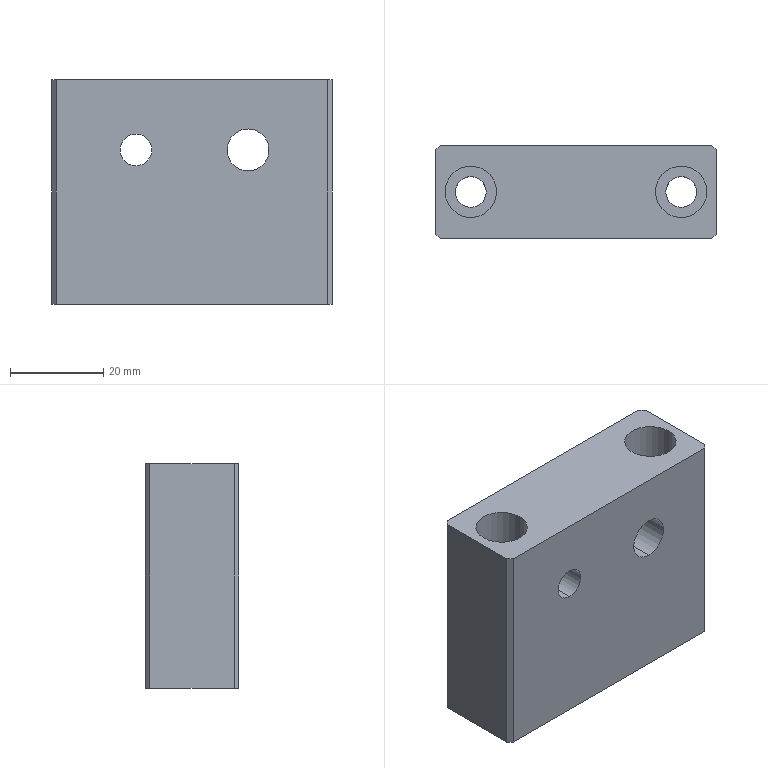Part | SolidWorks | features HoleWzd 3, Chamfer 1, Extrusion 1 | 1 solid | 24 faces | box 60 x 20 x 48 mm | volume 51248 mm3 | cylinder 12 | plane 12 | commonest cylinder face diameters 6.6 x4 11 x4 6.8 x2 9 x2
STEP:
#1=CARTESIAN_POINT('',(12.,10.,37.5));
#2=VERTEX_POINT('',#1);
#3=CARTESIAN_POINT('',(12.,10.,28.5));
#4=VERTEX_POINT('',#3);
#5=CARTESIAN_POINT('',(12.,10.,33.));
#6=DIRECTION('',(0.,-1.,0.));
#7=DIRECTION('',(0.,0.,-1.));
#8=AXIS2_PLACEMENT_3D('',#5,#6,#7);
#9=CIRCLE('',#8,4.5);
#10=EDGE_CURVE('',#2,#4,#9,.T.);
#11=ORIENTED_EDGE('',*,*,#10,.F.);
#12=CARTESIAN_POINT('',(12.,-10.,37.5));
#13=VERTEX_POINT('',#12);
#14=CARTESIAN_POINT('',(12.,-10.,37.5));
#15=DIRECTION('',(0.,-1.,0.));
#16=VECTOR('',#15,1000.);
#17=LINE('',#14,#16);
#18=EDGE_CURVE('',#2,#13,#17,.T.);
#19=ORIENTED_EDGE('',*,*,#18,.T.);
#20=CARTESIAN_POINT('',(12.,-10.,28.5));
#21=VERTEX_POINT('',#20);
#22=CARTESIAN_POINT('',(12.,-10.,33.));
#23=DIRECTION('',(0.,-1.,0.));
#24=DIRECTION('',(0.,0.,-1.));
#25=AXIS2_PLACEMENT_3D('',#22,#23,#24);
#26=CIRCLE('',#25,4.5);
#27=EDGE_CURVE('',#13,#21,#26,.T.);
#28=ORIENTED_EDGE('',*,*,#27,.T.);
#29=CARTESIAN_POINT('',(12.,-10.,28.5));
#30=DIRECTION('',(0.,-1.,0.));
#31=VECTOR('',#30,1000.);
#32=LINE('',#29,#31);
#33=EDGE_CURVE('',#4,#21,#32,.T.);
#34=ORIENTED_EDGE('',*,*,#33,.F.);
#35=EDGE_LOOP('',(#11,#19,#28,#34));
#36=FACE_OUTER_BOUND('',#35,.T.);
#37=CARTESIAN_POINT('',(12.,-10.,33.));
#38=DIRECTION('',(0.,-1.,0.));
#39=DIRECTION('',(0.,0.,-1.));
#40=AXIS2_PLACEMENT_3D('',#37,#38,#39);
#41=CYLINDRICAL_SURFACE('',#40,4.5);
#42=ADVANCED_FACE('',(#36),#41,.F.);
#43=CARTESIAN_POINT('',(-12.,10.,36.4));
#44=VERTEX_POINT('',#43);
#45=CARTESIAN_POINT('',(-12.,10.,29.6));
#46=VERTEX_POINT('',#45);
#47=CARTESIAN_POINT('',(-12.,10.,33.));
#48=DIRECTION('',(0.,-1.,0.));
#49=DIRECTION('',(0.,0.,-1.));
#50=AXIS2_PLACEMENT_3D('',#47,#48,#49);
#51=CIRCLE('',#50,3.4);
#52=EDGE_CURVE('',#44,#46,#51,.T.);
#53=ORIENTED_EDGE('',*,*,#52,.F.);
#54=CARTESIAN_POINT('',(-12.,-10.,36.4));
#55=VERTEX_POINT('',#54);
#56=CARTESIAN_POINT('',(-12.,-10.,36.4));
#57=DIRECTION('',(0.,-1.,0.));
#58=VECTOR('',#57,1000.);
#59=LINE('',#56,#58);
#60=EDGE_CURVE('',#44,#55,#59,.T.);
#61=ORIENTED_EDGE('',*,*,#60,.T.);
#62=CARTESIAN_POINT('',(-12.,-10.,29.6));
#63=VERTEX_POINT('',#62);
#64=CARTESIAN_POINT('',(-12.,-10.,33.));
#65=DIRECTION('',(0.,-1.,0.));
#66=DIRECTION('',(0.,0.,-1.));
#67=AXIS2_PLACEMENT_3D('',#64,#65,#66);
#68=CIRCLE('',#67,3.4);
#69=EDGE_CURVE('',#55,#63,#68,.T.);
#70=ORIENTED_EDGE('',*,*,#69,.T.);
#71=CARTESIAN_POINT('',(-12.,-10.,29.6));
#72=DIRECTION('',(0.,-1.,0.));
#73=VECTOR('',#72,1000.);
#74=LINE('',#71,#73);
#75=EDGE_CURVE('',#46,#63,#74,.T.);
#76=ORIENTED_EDGE('',*,*,#75,.F.);
#77=EDGE_LOOP('',(#53,#61,#70,#76));
#78=FACE_OUTER_BOUND('',#77,.T.);
#79=CARTESIAN_POINT('',(-12.,-10.,33.));
#80=DIRECTION('',(0.,-1.,0.));
#81=DIRECTION('',(0.,0.,-1.));
#82=AXIS2_PLACEMENT_3D('',#79,#80,#81);
#83=CYLINDRICAL_SURFACE('',#82,3.4);
#84=ADVANCED_FACE('',(#78),#83,.F.);
#85=CARTESIAN_POINT('',(-28.,0.,40.));
#86=VERTEX_POINT('',#85);
#87=CARTESIAN_POINT('',(-17.,0.,40.));
#88=VERTEX_POINT('',#87);
#89=CARTESIAN_POINT('',(-22.5,0.,40.));
#90=DIRECTION('',(0.,0.,1.));
#91=DIRECTION('',(1.,0.,0.));
#92=AXIS2_PLACEMENT_3D('',#89,#90,#91);
#93=CIRCLE('',#92,5.5);
#94=EDGE_CURVE('',#86,#88,#93,.T.);
#95=ORIENTED_EDGE('',*,*,#94,.F.);
#96=CARTESIAN_POINT('',(-28.,0.,48.));
#97=VERTEX_POINT('',#96);
#98=CARTESIAN_POINT('',(-28.,0.,48.));
#99=DIRECTION('',(0.,0.,1.));
#100=VECTOR('',#99,1000.);
#101=LINE('',#98,#100);
#102=EDGE_CURVE('',#86,#97,#101,.T.);
#103=ORIENTED_EDGE('',*,*,#102,.T.);
#104=CARTESIAN_POINT('',(-17.,0.,48.));
#105=VERTEX_POINT('',#104);
#106=CARTESIAN_POINT('',(-22.5,0.,48.));
#107=DIRECTION('',(0.,0.,1.));
#108=DIRECTION('',(1.,0.,0.));
#109=AXIS2_PLACEMENT_3D('',#106,#107,#108);
#110=CIRCLE('',#109,5.5);
#111=EDGE_CURVE('',#97,#105,#110,.T.);
#112=ORIENTED_EDGE('',*,*,#111,.T.);
#113=CARTESIAN_POINT('',(-17.,0.,48.));
#114=DIRECTION('',(0.,0.,1.));
#115=VECTOR('',#114,1000.);
#116=LINE('',#113,#115);
#117=EDGE_CURVE('',#88,#105,#116,.T.);
#118=ORIENTED_EDGE('',*,*,#117,.F.);
#119=EDGE_LOOP('',(#95,#103,#112,#118));
#120=FACE_OUTER_BOUND('',#119,.T.);
#121=CARTESIAN_POINT('',(-22.5,0.,48.));
#122=DIRECTION('',(0.,0.,1.));
#123=DIRECTION('',(1.,0.,0.));
#124=AXIS2_PLACEMENT_3D('',#121,#122,#123);
#125=CYLINDRICAL_SURFACE('',#124,5.5);
#126=ADVANCED_FACE('',(#120),#125,.F.);
#127=CARTESIAN_POINT('',(-25.8,0.,0.));
#128=VERTEX_POINT('',#127);
#129=CARTESIAN_POINT('',(-19.2,0.,0.));
#130=VERTEX_POINT('',#129);
#131=CARTESIAN_POINT('',(-22.5,0.,0.));
#132=DIRECTION('',(0.,0.,1.));
#133=DIRECTION('',(1.,0.,0.));
#134=AXIS2_PLACEMENT_3D('',#131,#132,#133);
#135=CIRCLE('',#134,3.3);
#136=EDGE_CURVE('',#128,#130,#135,.T.);
#137=ORIENTED_EDGE('',*,*,#136,.F.);
#138=CARTESIAN_POINT('',(-25.8,0.,40.));
#139=VERTEX_POINT('',#138);
#140=CARTESIAN_POINT('',(-25.8,0.,48.));
#141=DIRECTION('',(0.,0.,1.));
#142=VECTOR('',#141,1000.);
#143=LINE('',#140,#142);
#144=EDGE_CURVE('',#128,#139,#143,.T.);
#145=ORIENTED_EDGE('',*,*,#144,.T.);
#146=CARTESIAN_POINT('',(-19.2,0.,40.));
#147=VERTEX_POINT('',#146);
#148=CARTESIAN_POINT('',(-22.5,0.,40.));
#149=DIRECTION('',(0.,0.,1.));
#150=DIRECTION('',(1.,0.,0.));
#151=AXIS2_PLACEMENT_3D('',#148,#149,#150);
#152=CIRCLE('',#151,3.3);
#153=EDGE_CURVE('',#139,#147,#152,.T.);
#154=ORIENTED_EDGE('',*,*,#153,.T.);
#155=CARTESIAN_POINT('',(-19.2,0.,48.));
#156=DIRECTION('',(0.,0.,1.));
#157=VECTOR('',#156,1000.);
#158=LINE('',#155,#157);
#159=EDGE_CURVE('',#130,#147,#158,.T.);
#160=ORIENTED_EDGE('',*,*,#159,.F.);
#161=EDGE_LOOP('',(#137,#145,#154,#160));
#162=FACE_OUTER_BOUND('',#161,.T.);
#163=CARTESIAN_POINT('',(-22.5,0.,48.));
#164=DIRECTION('',(0.,0.,1.));
#165=DIRECTION('',(1.,0.,0.));
#166=AXIS2_PLACEMENT_3D('',#163,#164,#165);
#167=CYLINDRICAL_SURFACE('',#166,3.3);
#168=ADVANCED_FACE('',(#162),#167,.F.);
#169=CARTESIAN_POINT('',(17.,0.,40.));
#170=VERTEX_POINT('',#169);
#171=CARTESIAN_POINT('',(28.,0.,40.));
#172=VERTEX_POINT('',#171);
#173=CARTESIAN_POINT('',(22.5,0.,40.));
#174=DIRECTION('',(0.,0.,1.));
#175=DIRECTION('',(1.,0.,0.));
#176=AXIS2_PLACEMENT_3D('',#173,#174,#175);
#177=CIRCLE('',#176,5.5);
#178=EDGE_CURVE('',#170,#172,#177,.T.);
#179=ORIENTED_EDGE('',*,*,#178,.F.);
#180=CARTESIAN_POINT('',(17.,0.,48.));
#181=VERTEX_POINT('',#180);
#182=CARTESIAN_POINT('',(17.,0.,48.));
#183=DIRECTION('',(0.,0.,1.));
#184=VECTOR('',#183,1000.);
#185=LINE('',#182,#184);
#186=EDGE_CURVE('',#170,#181,#185,.T.);
#187=ORIENTED_EDGE('',*,*,#186,.T.);
#188=CARTESIAN_POINT('',(28.,0.,48.));
#189=VERTEX_POINT('',#188);
#190=CARTESIAN_POINT('',(22.5,0.,48.));
#191=DIRECTION('',(0.,0.,1.));
#192=DIRECTION('',(1.,0.,0.));
#193=AXIS2_PLACEMENT_3D('',#190,#191,#192);
#194=CIRCLE('',#193,5.5);
#195=EDGE_CURVE('',#181,#189,#194,.T.);
#196=ORIENTED_EDGE('',*,*,#195,.T.);
#197=CARTESIAN_POINT('',(28.,0.,48.));
#198=DIRECTION('',(0.,0.,1.));
#199=VECTOR('',#198,1000.);
#200=LINE('',#197,#199);
#201=EDGE_CURVE('',#172,#189,#200,.T.);
#202=ORIENTED_EDGE('',*,*,#201,.F.);
#203=EDGE_LOOP('',(#179,#187,#196,#202));
#204=FACE_OUTER_BOUND('',#203,.T.);
#205=CARTESIAN_POINT('',(22.5,0.,48.));
#206=DIRECTION('',(0.,0.,1.));
#207=DIRECTION('',(1.,0.,0.));
#208=AXIS2_PLACEMENT_3D('',#205,#206,#207);
#209=CYLINDRICAL_SURFACE('',#208,5.5);
#210=ADVANCED_FACE('',(#204),#209,.F.);
#211=CARTESIAN_POINT('',(19.2,0.,0.));
#212=VERTEX_POINT('',#211);
#213=CARTESIAN_POINT('',(25.8,0.,0.));
#214=VERTEX_POINT('',#213);
#215=CARTESIAN_POINT('',(22.5,0.,0.));
#216=DIRECTION('',(0.,0.,1.));
#217=DIRECTION('',(1.,0.,0.));
#218=AXIS2_PLACEMENT_3D('',#215,#216,#217);
#219=CIRCLE('',#218,3.3);
#220=EDGE_CURVE('',#212,#214,#219,.T.);
#221=ORIENTED_EDGE('',*,*,#220,.F.);
#222=CARTESIAN_POINT('',(19.2,0.,40.));
#223=VERTEX_POINT('',#222);
#224=CARTESIAN_POINT('',(19.2,0.,48.));
#225=DIRECTION('',(0.,0.,1.));
#226=VECTOR('',#225,1000.);
#227=LINE('',#224,#226);
#228=EDGE_CURVE('',#212,#223,#227,.T.);
#229=ORIENTED_EDGE('',*,*,#228,.T.);
#230=CARTESIAN_POINT('',(25.8,0.,40.));
#231=VERTEX_POINT('',#230);
#232=CARTESIAN_POINT('',(22.5,0.,40.));
#233=DIRECTION('',(0.,0.,1.));
#234=DIRECTION('',(1.,0.,0.));
#235=AXIS2_PLACEMENT_3D('',#232,#233,#234);
#236=CIRCLE('',#235,3.3);
#237=EDGE_CURVE('',#223,#231,#236,.T.);
#238=ORIENTED_EDGE('',*,*,#237,.T.);
#239=CARTESIAN_POINT('',(25.8,0.,48.));
#240=DIRECTION('',(0.,0.,1.));
#241=VECTOR('',#240,1000.);
#242=LINE('',#239,#241);
#243=EDGE_CURVE('',#214,#231,#242,.T.);
#244=ORIENTED_EDGE('',*,*,#243,.F.);
#245=EDGE_LOOP('',(#221,#229,#238,#244));
#246=FACE_OUTER_BOUND('',#245,.T.);
#247=CARTESIAN_POINT('',(22.5,0.,48.));
#248=DIRECTION('',(0.,0.,1.));
#249=DIRECTION('',(1.,0.,0.));
#250=AXIS2_PLACEMENT_3D('',#247,#248,#249);
#251=CYLINDRICAL_SURFACE('',#250,3.3);
#252=ADVANCED_FACE('',(#246),#251,.F.);
#253=CARTESIAN_POINT('',(-12.,-10.,33.));
#254=DIRECTION('',(0.,-1.,0.));
#255=DIRECTION('',(0.,0.,-1.));
#256=AXIS2_PLACEMENT_3D('',#253,#254,#255);
#257=CIRCLE('',#256,3.4);
#258=EDGE_CURVE('',#63,#55,#257,.T.);
#259=ORIENTED_EDGE('',*,*,#258,.F.);
#260=ORIENTED_EDGE('',*,*,#69,.F.);
#261=EDGE_LOOP('',(#259,#260));
#262=FACE_BOUND('',#261,.T.);
#263=CARTESIAN_POINT('',(-29.,-10.,0.));
#264=VERTEX_POINT('',#263);
#265=CARTESIAN_POINT('',(29.,-10.,0.));
#266=VERTEX_POINT('',#265);
#267=CARTESIAN_POINT('',(-30.,-10.,0.));
#268=DIRECTION('',(1.,0.,0.));
#269=VECTOR('',#268,1000.);
#270=LINE('',#267,#269);
#271=EDGE_CURVE('',#264,#266,#270,.T.);
#272=ORIENTED_EDGE('',*,*,#271,.T.);
#273=CARTESIAN_POINT('',(29.,-10.,48.));
#274=VERTEX_POINT('',#273);
#275=CARTESIAN_POINT('',(29.,-10.,48.));
#276=DIRECTION('',(0.,0.,1.));
#277=VECTOR('',#276,1000.);
#278=LINE('',#275,#277);
#279=EDGE_CURVE('',#266,#274,#278,.T.);
#280=ORIENTED_EDGE('',*,*,#279,.T.);
#281=CARTESIAN_POINT('',(-29.,-10.,48.));
#282=VERTEX_POINT('',#281);
#283=CARTESIAN_POINT('',(-30.,-10.,48.));
#284=DIRECTION('',(1.,0.,0.));
#285=VECTOR('',#284,1000.);
#286=LINE('',#283,#285);
#287=EDGE_CURVE('',#282,#274,#286,.T.);
#288=ORIENTED_EDGE('',*,*,#287,.F.);
#289=CARTESIAN_POINT('',(-29.,-10.,48.));
#290=DIRECTION('',(0.,0.,-1.));
#291=VECTOR('',#290,1000.);
#292=LINE('',#289,#291);
#293=EDGE_CURVE('',#282,#264,#292,.T.);
#294=ORIENTED_EDGE('',*,*,#293,.T.);
#295=EDGE_LOOP('',(#272,#280,#288,#294));
#296=FACE_OUTER_BOUND('',#295,.T.);
#297=CARTESIAN_POINT('',(12.,-10.,33.));
#298=DIRECTION('',(0.,-1.,0.));
#299=DIRECTION('',(0.,0.,-1.));
#300=AXIS2_PLACEMENT_3D('',#297,#298,#299);
#301=CIRCLE('',#300,4.5);
#302=EDGE_CURVE('',#21,#13,#301,.T.);
#303=ORIENTED_EDGE('',*,*,#302,.F.);
#304=ORIENTED_EDGE('',*,*,#27,.F.);
#305=EDGE_LOOP('',(#303,#304));
#306=FACE_BOUND('',#305,.T.);
#307=CARTESIAN_POINT('',(-30.,-10.,48.));
#308=DIRECTION('',(0.,1.,0.));
#309=DIRECTION('',(0.,0.,1.));
#310=AXIS2_PLACEMENT_3D('',#307,#308,#309);
#311=PLANE('',#310);
#312=ADVANCED_FACE('',(#262,#296,#306),#311,.F.);
#313=CARTESIAN_POINT('',(30.,-9.,0.));
#314=VERTEX_POINT('',#313);
#315=CARTESIAN_POINT('',(30.,9.,0.));
#316=VERTEX_POINT('',#315);
#317=CARTESIAN_POINT('',(30.,10.,0.));
#318=DIRECTION('',(0.,1.,0.));
#319=VECTOR('',#318,1000.);
#320=LINE('',#317,#319);
#321=EDGE_CURVE('',#314,#316,#320,.T.);
#322=ORIENTED_EDGE('',*,*,#321,.T.);
#323=CARTESIAN_POINT('',(30.,9.,48.));
#324=VERTEX_POINT('',#323);
#325=CARTESIAN_POINT('',(30.,9.,48.));
#326=DIRECTION('',(0.,0.,1.));
#327=VECTOR('',#326,1000.);
#328=LINE('',#325,#327);
#329=EDGE_CURVE('',#316,#324,#328,.T.);
#330=ORIENTED_EDGE('',*,*,#329,.T.);
#331=CARTESIAN_POINT('',(30.,-9.,48.));
#332=VERTEX_POINT('',#331);
#333=CARTESIAN_POINT('',(30.,10.,48.));
#334=DIRECTION('',(0.,1.,0.));
#335=VECTOR('',#334,1000.);
#336=LINE('',#333,#335);
#337=EDGE_CURVE('',#332,#324,#336,.T.);
#338=ORIENTED_EDGE('',*,*,#337,.F.);
#339=CARTESIAN_POINT('',(30.,-9.,48.));
#340=DIRECTION('',(0.,0.,-1.));
#341=VECTOR('',#340,1000.);
#342=LINE('',#339,#341);
#343=EDGE_CURVE('',#332,#314,#342,.T.);
#344=ORIENTED_EDGE('',*,*,#343,.T.);
#345=EDGE_LOOP('',(#322,#330,#338,#344));
#346=FACE_OUTER_BOUND('',#345,.T.);
#347=CARTESIAN_POINT('',(30.,10.,48.));
#348=DIRECTION('',(-1.,0.,0.));
#349=DIRECTION('',(0.,-1.,0.));
#350=AXIS2_PLACEMENT_3D('',#347,#348,#349);
#351=PLANE('',#350);
#352=ADVANCED_FACE('',(#346),#351,.F.);
#353=CARTESIAN_POINT('',(12.,10.,33.));
#354=DIRECTION('',(0.,-1.,0.));
#355=DIRECTION('',(0.,0.,-1.));
#356=AXIS2_PLACEMENT_3D('',#353,#354,#355);
#357=CIRCLE('',#356,4.5);
#358=EDGE_CURVE('',#4,#2,#357,.T.);
#359=ORIENTED_EDGE('',*,*,#358,.T.);
#360=ORIENTED_EDGE('',*,*,#10,.T.);
#361=EDGE_LOOP('',(#359,#360));
#362=FACE_BOUND('',#361,.T.);
#363=CARTESIAN_POINT('',(-12.,10.,33.));
#364=DIRECTION('',(0.,-1.,0.));
#365=DIRECTION('',(0.,0.,-1.));
#366=AXIS2_PLACEMENT_3D('',#363,#364,#365);
#367=CIRCLE('',#366,3.4);
#368=EDGE_CURVE('',#46,#44,#367,.T.);
#369=ORIENTED_EDGE('',*,*,#368,.T.);
#370=ORIENTED_EDGE('',*,*,#52,.T.);
#371=EDGE_LOOP('',(#369,#370));
#372=FACE_BOUND('',#371,.T.);
#373=CARTESIAN_POINT('',(29.,10.,48.));
#374=VERTEX_POINT('',#373);
#375=CARTESIAN_POINT('',(-29.,10.,48.));
#376=VERTEX_POINT('',#375);
#377=CARTESIAN_POINT('',(-30.,10.,48.));
#378=DIRECTION('',(-1.,0.,0.));
#379=VECTOR('',#378,1000.);
#380=LINE('',#377,#379);
#381=EDGE_CURVE('',#374,#376,#380,.T.);
#382=ORIENTED_EDGE('',*,*,#381,.F.);
#383=CARTESIAN_POINT('',(29.,10.,0.));
#384=VERTEX_POINT('',#383);
#385=CARTESIAN_POINT('',(29.,10.,48.));
#386=DIRECTION('',(0.,0.,-1.));
#387=VECTOR('',#386,1000.);
#388=LINE('',#385,#387);
#389=EDGE_CURVE('',#374,#384,#388,.T.);
#390=ORIENTED_EDGE('',*,*,#389,.T.);
#391=CARTESIAN_POINT('',(-29.,10.,0.));
#392=VERTEX_POINT('',#391);
#393=CARTESIAN_POINT('',(-30.,10.,0.));
#394=DIRECTION('',(-1.,0.,0.));
#395=VECTOR('',#394,1000.);
#396=LINE('',#393,#395);
#397=EDGE_CURVE('',#384,#392,#396,.T.);
#398=ORIENTED_EDGE('',*,*,#397,.T.);
#399=CARTESIAN_POINT('',(-29.,10.,48.));
#400=DIRECTION('',(0.,0.,1.));
#401=VECTOR('',#400,1000.);
#402=LINE('',#399,#401);
#403=EDGE_CURVE('',#392,#376,#402,.T.);
#404=ORIENTED_EDGE('',*,*,#403,.T.);
#405=EDGE_LOOP('',(#382,#390,#398,#404));
#406=FACE_OUTER_BOUND('',#405,.T.);
#407=CARTESIAN_POINT('',(-30.,10.,48.));
#408=DIRECTION('',(0.,-1.,0.));
#409=DIRECTION('',(0.,0.,-1.));
#410=AXIS2_PLACEMENT_3D('',#407,#408,#409);
#411=PLANE('',#410);
#412=ADVANCED_FACE('',(#362,#372,#406),#411,.F.);
#413=CARTESIAN_POINT('',(-30.,9.,48.));
#414=VERTEX_POINT('',#413);
#415=CARTESIAN_POINT('',(-30.,-9.,48.));
#416=VERTEX_POINT('',#415);
#417=CARTESIAN_POINT('',(-30.,10.,48.));
#418=DIRECTION('',(0.,-1.,0.));
#419=VECTOR('',#418,1000.);
#420=LINE('',#417,#419);
#421=EDGE_CURVE('',#414,#416,#420,.T.);
#422=ORIENTED_EDGE('',*,*,#421,.F.);
#423=CARTESIAN_POINT('',(-30.,9.,0.));
#424=VERTEX_POINT('',#423);
#425=CARTESIAN_POINT('',(-30.,9.,48.));
#426=DIRECTION('',(0.,0.,-1.));
#427=VECTOR('',#426,1000.);
#428=LINE('',#425,#427);
#429=EDGE_CURVE('',#414,#424,#428,.T.);
#430=ORIENTED_EDGE('',*,*,#429,.T.);
#431=CARTESIAN_POINT('',(-30.,-9.,0.));
#432=VERTEX_POINT('',#431);
#433=CARTESIAN_POINT('',(-30.,10.,0.));
#434=DIRECTION('',(0.,-1.,0.));
#435=VECTOR('',#434,1000.);
#436=LINE('',#433,#435);
#437=EDGE_CURVE('',#424,#432,#436,.T.);
#438=ORIENTED_EDGE('',*,*,#437,.T.);
#439=CARTESIAN_POINT('',(-30.,-9.,48.));
#440=DIRECTION('',(0.,0.,1.));
#441=VECTOR('',#440,1000.);
#442=LINE('',#439,#441);
#443=EDGE_CURVE('',#432,#416,#442,.T.);
#444=ORIENTED_EDGE('',*,*,#443,.T.);
#445=EDGE_LOOP('',(#422,#430,#438,#444));
#446=FACE_OUTER_BOUND('',#445,.T.);
#447=CARTESIAN_POINT('',(-30.,10.,48.));
#448=DIRECTION('',(1.,0.,0.));
#449=DIRECTION('',(0.,1.,0.));
#450=AXIS2_PLACEMENT_3D('',#447,#448,#449);
#451=PLANE('',#450);
#452=ADVANCED_FACE('',(#446),#451,.F.);
#453=CARTESIAN_POINT('',(-22.5,0.,48.));
#454=DIRECTION('',(0.,0.,1.));
#455=DIRECTION('',(1.,0.,0.));
#456=AXIS2_PLACEMENT_3D('',#453,#454,#455);
#457=CIRCLE('',#456,5.5);
#458=EDGE_CURVE('',#105,#97,#457,.T.);
#459=ORIENTED_EDGE('',*,*,#458,.F.);
#460=ORIENTED_EDGE('',*,*,#111,.F.);
#461=EDGE_LOOP('',(#459,#460));
#462=FACE_BOUND('',#461,.T.);
#463=CARTESIAN_POINT('',(22.5,0.,48.));
#464=DIRECTION('',(0.,0.,1.));
#465=DIRECTION('',(1.,0.,0.));
#466=AXIS2_PLACEMENT_3D('',#463,#464,#465);
#467=CIRCLE('',#466,5.5);
#468=EDGE_CURVE('',#189,#181,#467,.T.);
#469=ORIENTED_EDGE('',*,*,#468,.F.);
#470=ORIENTED_EDGE('',*,*,#195,.F.);
#471=EDGE_LOOP('',(#469,#470));
#472=FACE_BOUND('',#471,.T.);
#473=ORIENTED_EDGE('',*,*,#337,.T.);
#474=CARTESIAN_POINT('',(19.5,19.5,48.));
#475=DIRECTION('',(-0.7071,0.7071,0.));
#476=VECTOR('',#475,1000.);
#477=LINE('',#474,#476);
#478=EDGE_CURVE('',#324,#374,#477,.T.);
#479=ORIENTED_EDGE('',*,*,#478,.T.);
#480=ORIENTED_EDGE('',*,*,#381,.T.);
#481=CARTESIAN_POINT('',(-19.5,19.5,48.));
#482=DIRECTION('',(-0.7071,-0.7071,0.));
#483=VECTOR('',#482,1000.);
#484=LINE('',#481,#483);
#485=EDGE_CURVE('',#376,#414,#484,.T.);
#486=ORIENTED_EDGE('',*,*,#485,.T.);
#487=ORIENTED_EDGE('',*,*,#421,.T.);
#488=CARTESIAN_POINT('',(-19.5,-19.5,48.));
#489=DIRECTION('',(0.7071,-0.7071,0.));
#490=VECTOR('',#489,1000.);
#491=LINE('',#488,#490);
#492=EDGE_CURVE('',#416,#282,#491,.T.);
#493=ORIENTED_EDGE('',*,*,#492,.T.);
#494=ORIENTED_EDGE('',*,*,#287,.T.);
#495=CARTESIAN_POINT('',(19.5,-19.5,48.));
#496=DIRECTION('',(0.7071,0.7071,0.));
#497=VECTOR('',#496,1000.);
#498=LINE('',#495,#497);
#499=EDGE_CURVE('',#274,#332,#498,.T.);
#500=ORIENTED_EDGE('',*,*,#499,.T.);
#501=EDGE_LOOP('',(#473,#479,#480,#486,#487,#493,#494,#500));
#502=FACE_OUTER_BOUND('',#501,.T.);
#503=CARTESIAN_POINT('',(0.,0.,48.));
#504=DIRECTION('',(0.,0.,1.));
#505=DIRECTION('',(1.,0.,0.));
#506=AXIS2_PLACEMENT_3D('',#503,#504,#505);
#507=PLANE('',#506);
#508=ADVANCED_FACE('',(#462,#472,#502),#507,.T.);
#509=CARTESIAN_POINT('',(-22.5,0.,0.));
#510=DIRECTION('',(0.,0.,1.));
#511=DIRECTION('',(1.,0.,0.));
#512=AXIS2_PLACEMENT_3D('',#509,#510,#511);
#513=CIRCLE('',#512,3.3);
#514=EDGE_CURVE('',#130,#128,#513,.T.);
#515=ORIENTED_EDGE('',*,*,#514,.T.);
#516=ORIENTED_EDGE('',*,*,#136,.T.);
#517=EDGE_LOOP('',(#515,#516));
#518=FACE_BOUND('',#517,.T.);
#519=CARTESIAN_POINT('',(22.5,0.,0.));
#520=DIRECTION('',(0.,0.,1.));
#521=DIRECTION('',(1.,0.,0.));
#522=AXIS2_PLACEMENT_3D('',#519,#520,#521);
#523=CIRCLE('',#522,3.3);
#524=EDGE_CURVE('',#214,#212,#523,.T.);
#525=ORIENTED_EDGE('',*,*,#524,.T.);
#526=ORIENTED_EDGE('',*,*,#220,.T.);
#527=EDGE_LOOP('',(#525,#526));
#528=FACE_BOUND('',#527,.T.);
#529=ORIENTED_EDGE('',*,*,#397,.F.);
#530=CARTESIAN_POINT('',(29.,10.,0.));
#531=DIRECTION('',(0.7071,-0.7071,0.));
#532=VECTOR('',#531,1000.);
#533=LINE('',#530,#532);
#534=EDGE_CURVE('',#384,#316,#533,.T.);
#535=ORIENTED_EDGE('',*,*,#534,.T.);
#536=ORIENTED_EDGE('',*,*,#321,.F.);
#537=CARTESIAN_POINT('',(30.,-9.,0.));
#538=DIRECTION('',(-0.7071,-0.7071,0.));
#539=VECTOR('',#538,1000.);
#540=LINE('',#537,#539);
#541=EDGE_CURVE('',#314,#266,#540,.T.);
#542=ORIENTED_EDGE('',*,*,#541,.T.);
#543=ORIENTED_EDGE('',*,*,#271,.F.);
#544=CARTESIAN_POINT('',(-29.,-10.,0.));
#545=DIRECTION('',(-0.7071,0.7071,0.));
#546=VECTOR('',#545,1000.);
#547=LINE('',#544,#546);
#548=EDGE_CURVE('',#264,#432,#547,.T.);
#549=ORIENTED_EDGE('',*,*,#548,.T.);
#550=ORIENTED_EDGE('',*,*,#437,.F.);
#551=CARTESIAN_POINT('',(-30.,9.,0.));
#552=DIRECTION('',(0.7071,0.7071,0.));
#553=VECTOR('',#552,1000.);
#554=LINE('',#551,#553);
#555=EDGE_CURVE('',#424,#392,#554,.T.);
#556=ORIENTED_EDGE('',*,*,#555,.T.);
#557=EDGE_LOOP('',(#529,#535,#536,#542,#543,#549,#550,#556));
#558=FACE_OUTER_BOUND('',#557,.T.);
#559=CARTESIAN_POINT('',(0.,0.,0.));
#560=DIRECTION('',(0.,0.,1.));
#561=DIRECTION('',(1.,0.,0.));
#562=AXIS2_PLACEMENT_3D('',#559,#560,#561);
#563=PLANE('',#562);
#564=ADVANCED_FACE('',(#518,#528,#558),#563,.F.);
#565=ORIENTED_EDGE('',*,*,#228,.F.);
#566=ORIENTED_EDGE('',*,*,#524,.F.);
#567=ORIENTED_EDGE('',*,*,#243,.T.);
#568=CARTESIAN_POINT('',(22.5,0.,40.));
#569=DIRECTION('',(0.,0.,1.));
#570=DIRECTION('',(1.,0.,0.));
#571=AXIS2_PLACEMENT_3D('',#568,#569,#570);
#572=CIRCLE('',#571,3.3);
#573=EDGE_CURVE('',#231,#223,#572,.T.);
#574=ORIENTED_EDGE('',*,*,#573,.T.);
#575=EDGE_LOOP('',(#565,#566,#567,#574));
#576=FACE_OUTER_BOUND('',#575,.T.);
#577=CARTESIAN_POINT('',(22.5,0.,48.));
#578=DIRECTION('',(0.,0.,1.));
#579=DIRECTION('',(1.,0.,0.));
#580=AXIS2_PLACEMENT_3D('',#577,#578,#579);
#581=CYLINDRICAL_SURFACE('',#580,3.3);
#582=ADVANCED_FACE('',(#576),#581,.F.);
#583=ORIENTED_EDGE('',*,*,#573,.F.);
#584=ORIENTED_EDGE('',*,*,#237,.F.);
#585=EDGE_LOOP('',(#583,#584));
#586=FACE_BOUND('',#585,.T.);
#587=CARTESIAN_POINT('',(22.5,0.,40.));
#588=DIRECTION('',(0.,0.,1.));
#589=DIRECTION('',(1.,0.,0.));
#590=AXIS2_PLACEMENT_3D('',#587,#588,#589);
#591=CIRCLE('',#590,5.5);
#592=EDGE_CURVE('',#172,#170,#591,.T.);
#593=ORIENTED_EDGE('',*,*,#592,.T.);
#594=ORIENTED_EDGE('',*,*,#178,.T.);
#595=EDGE_LOOP('',(#593,#594));
#596=FACE_OUTER_BOUND('',#595,.T.);
#597=CARTESIAN_POINT('',(25.8,0.,40.));
#598=DIRECTION('',(0.,0.,-1.));
#599=DIRECTION('',(-1.,0.,0.));
#600=AXIS2_PLACEMENT_3D('',#597,#598,#599);
#601=PLANE('',#600);
#602=ADVANCED_FACE('',(#586,#596),#601,.F.);
#603=ORIENTED_EDGE('',*,*,#186,.F.);
#604=ORIENTED_EDGE('',*,*,#592,.F.);
#605=ORIENTED_EDGE('',*,*,#201,.T.);
#606=ORIENTED_EDGE('',*,*,#468,.T.);
#607=EDGE_LOOP('',(#603,#604,#605,#606));
#608=FACE_OUTER_BOUND('',#607,.T.);
#609=CARTESIAN_POINT('',(22.5,0.,48.));
#610=DIRECTION('',(0.,0.,1.));
#611=DIRECTION('',(1.,0.,0.));
#612=AXIS2_PLACEMENT_3D('',#609,#610,#611);
#613=CYLINDRICAL_SURFACE('',#612,5.5);
#614=ADVANCED_FACE('',(#608),#613,.F.);
#615=ORIENTED_EDGE('',*,*,#144,.F.);
#616=ORIENTED_EDGE('',*,*,#514,.F.);
#617=ORIENTED_EDGE('',*,*,#159,.T.);
#618=CARTESIAN_POINT('',(-22.5,0.,40.));
#619=DIRECTION('',(0.,0.,1.));
#620=DIRECTION('',(1.,0.,0.));
#621=AXIS2_PLACEMENT_3D('',#618,#619,#620);
#622=CIRCLE('',#621,3.3);
#623=EDGE_CURVE('',#147,#139,#622,.T.);
#624=ORIENTED_EDGE('',*,*,#623,.T.);
#625=EDGE_LOOP('',(#615,#616,#617,#624));
#626=FACE_OUTER_BOUND('',#625,.T.);
#627=CARTESIAN_POINT('',(-22.5,0.,48.));
#628=DIRECTION('',(0.,0.,1.));
#629=DIRECTION('',(1.,0.,0.));
#630=AXIS2_PLACEMENT_3D('',#627,#628,#629);
#631=CYLINDRICAL_SURFACE('',#630,3.3);
#632=ADVANCED_FACE('',(#626),#631,.F.);
#633=ORIENTED_EDGE('',*,*,#623,.F.);
#634=ORIENTED_EDGE('',*,*,#153,.F.);
#635=EDGE_LOOP('',(#633,#634));
#636=FACE_BOUND('',#635,.T.);
#637=CARTESIAN_POINT('',(-22.5,0.,40.));
#638=DIRECTION('',(0.,0.,1.));
#639=DIRECTION('',(1.,0.,0.));
#640=AXIS2_PLACEMENT_3D('',#637,#638,#639);
#641=CIRCLE('',#640,5.5);
#642=EDGE_CURVE('',#88,#86,#641,.T.);
#643=ORIENTED_EDGE('',*,*,#642,.T.);
#644=ORIENTED_EDGE('',*,*,#94,.T.);
#645=EDGE_LOOP('',(#643,#644));
#646=FACE_OUTER_BOUND('',#645,.T.);
#647=CARTESIAN_POINT('',(-19.2,0.,40.));
#648=DIRECTION('',(0.,0.,-1.));
#649=DIRECTION('',(-1.,0.,0.));
#650=AXIS2_PLACEMENT_3D('',#647,#648,#649);
#651=PLANE('',#650);
#652=ADVANCED_FACE('',(#636,#646),#651,.F.);
#653=ORIENTED_EDGE('',*,*,#102,.F.);
#654=ORIENTED_EDGE('',*,*,#642,.F.);
#655=ORIENTED_EDGE('',*,*,#117,.T.);
#656=ORIENTED_EDGE('',*,*,#458,.T.);
#657=EDGE_LOOP('',(#653,#654,#655,#656));
#658=FACE_OUTER_BOUND('',#657,.T.);
#659=CARTESIAN_POINT('',(-22.5,0.,48.));
#660=DIRECTION('',(0.,0.,1.));
#661=DIRECTION('',(1.,0.,0.));
#662=AXIS2_PLACEMENT_3D('',#659,#660,#661);
#663=CYLINDRICAL_SURFACE('',#662,5.5);
#664=ADVANCED_FACE('',(#658),#663,.F.);
#665=ORIENTED_EDGE('',*,*,#60,.F.);
#666=ORIENTED_EDGE('',*,*,#368,.F.);
#667=ORIENTED_EDGE('',*,*,#75,.T.);
#668=ORIENTED_EDGE('',*,*,#258,.T.);
#669=EDGE_LOOP('',(#665,#666,#667,#668));
#670=FACE_OUTER_BOUND('',#669,.T.);
#671=CARTESIAN_POINT('',(-12.,-10.,33.));
#672=DIRECTION('',(0.,-1.,0.));
#673=DIRECTION('',(0.,0.,-1.));
#674=AXIS2_PLACEMENT_3D('',#671,#672,#673);
#675=CYLINDRICAL_SURFACE('',#674,3.4);
#676=ADVANCED_FACE('',(#670),#675,.F.);
#677=ORIENTED_EDGE('',*,*,#18,.F.);
#678=ORIENTED_EDGE('',*,*,#358,.F.);
#679=ORIENTED_EDGE('',*,*,#33,.T.);
#680=ORIENTED_EDGE('',*,*,#302,.T.);
#681=EDGE_LOOP('',(#677,#678,#679,#680));
#682=FACE_OUTER_BOUND('',#681,.T.);
#683=CARTESIAN_POINT('',(12.,-10.,33.));
#684=DIRECTION('',(0.,-1.,0.));
#685=DIRECTION('',(0.,0.,-1.));
#686=AXIS2_PLACEMENT_3D('',#683,#684,#685);
#687=CYLINDRICAL_SURFACE('',#686,4.5);
#688=ADVANCED_FACE('',(#682),#687,.F.);
#689=ORIENTED_EDGE('',*,*,#478,.F.);
#690=ORIENTED_EDGE('',*,*,#329,.F.);
#691=ORIENTED_EDGE('',*,*,#534,.F.);
#692=ORIENTED_EDGE('',*,*,#389,.F.);
#693=EDGE_LOOP('',(#689,#690,#691,#692));
#694=FACE_OUTER_BOUND('',#693,.T.);
#695=CARTESIAN_POINT('',(29.,10.,48.));
#696=DIRECTION('',(-0.7071,-0.7071,0.));
#697=DIRECTION('',(0.,0.,-1.));
#698=AXIS2_PLACEMENT_3D('',#695,#696,#697);
#699=PLANE('',#698);
#700=ADVANCED_FACE('',(#694),#699,.F.);
#701=ORIENTED_EDGE('',*,*,#499,.F.);
#702=ORIENTED_EDGE('',*,*,#279,.F.);
#703=ORIENTED_EDGE('',*,*,#541,.F.);
#704=ORIENTED_EDGE('',*,*,#343,.F.);
#705=EDGE_LOOP('',(#701,#702,#703,#704));
#706=FACE_OUTER_BOUND('',#705,.T.);
#707=CARTESIAN_POINT('',(30.,-9.,48.));
#708=DIRECTION('',(-0.7071,0.7071,0.));
#709=DIRECTION('',(0.,0.,-1.));
#710=AXIS2_PLACEMENT_3D('',#707,#708,#709);
#711=PLANE('',#710);
#712=ADVANCED_FACE('',(#706),#711,.F.);
#713=ORIENTED_EDGE('',*,*,#485,.F.);
#714=ORIENTED_EDGE('',*,*,#403,.F.);
#715=ORIENTED_EDGE('',*,*,#555,.F.);
#716=ORIENTED_EDGE('',*,*,#429,.F.);
#717=EDGE_LOOP('',(#713,#714,#715,#716));
#718=FACE_OUTER_BOUND('',#717,.T.);
#719=CARTESIAN_POINT('',(-30.,9.,48.));
#720=DIRECTION('',(0.7071,-0.7071,0.));
#721=DIRECTION('',(0.,0.,-1.));
#722=AXIS2_PLACEMENT_3D('',#719,#720,#721);
#723=PLANE('',#722);
#724=ADVANCED_FACE('',(#718),#723,.F.);
#725=ORIENTED_EDGE('',*,*,#492,.F.);
#726=ORIENTED_EDGE('',*,*,#443,.F.);
#727=ORIENTED_EDGE('',*,*,#548,.F.);
#728=ORIENTED_EDGE('',*,*,#293,.F.);
#729=EDGE_LOOP('',(#725,#726,#727,#728));
#730=FACE_OUTER_BOUND('',#729,.T.);
#731=CARTESIAN_POINT('',(-29.,-10.,48.));
#732=DIRECTION('',(0.7071,0.7071,0.));
#733=DIRECTION('',(0.,0.,-1.));
#734=AXIS2_PLACEMENT_3D('',#731,#732,#733);
#735=PLANE('',#734);
#736=ADVANCED_FACE('',(#730),#735,.F.);
#737=CLOSED_SHELL('',(#42,#84,#126,#168,#210,#252,#312,#352,#412,#452,#508,#564,#582,#602,#614,#632,#652,#664,#676,#688,#700,#712,#724,#736));
#738=MANIFOLD_SOLID_BREP('',#737);
#739=CARTESIAN_POINT('',(0.,0.,0.));
#740=DIRECTION('',(0.,0.,1.));
#741=DIRECTION('',(1.,0.,0.));
#742=AXIS2_PLACEMENT_3D('',#739,#740,#741);
#743=(LENGTH_UNIT()NAMED_UNIT(*)SI_UNIT(.MILLI.,.METRE.));
#744=UNCERTAINTY_MEASURE_WITH_UNIT(LENGTH_MEASURE(0.00001),#743,'','');
#745=(NAMED_UNIT(*)PLANE_ANGLE_UNIT()SI_UNIT($,.RADIAN.));
#746=(NAMED_UNIT(*)SI_UNIT($,.STERADIAN.)SOLID_ANGLE_UNIT());
#747=(GEOMETRIC_REPRESENTATION_CONTEXT(3)GLOBAL_UNCERTAINTY_ASSIGNED_CONTEXT((#744))GLOBAL_UNIT_ASSIGNED_CONTEXT((#743,#745,#746))REPRESENTATION_CONTEXT('',''));
#748=ADVANCED_BREP_SHAPE_REPRESENTATION('',(#738,#742),#747);